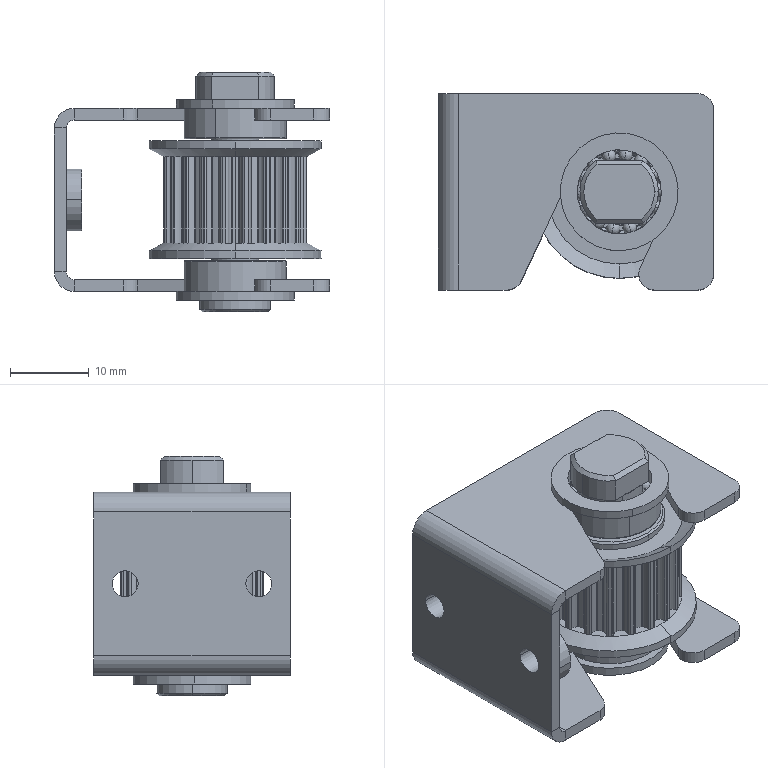Part | SolidWorks | 38 solids | 948 faces | box 35 x 25 x 30.5 mm | volume 7521 mm3 | cylinder 304 | sphere 304 | torus 184 | plane 127 | cone 25 | spline 4 | commonest cylinder face diameters 0.56 x54 0.3 x44 3.95 x42 4 x34 16.12 x21 18.34 x20